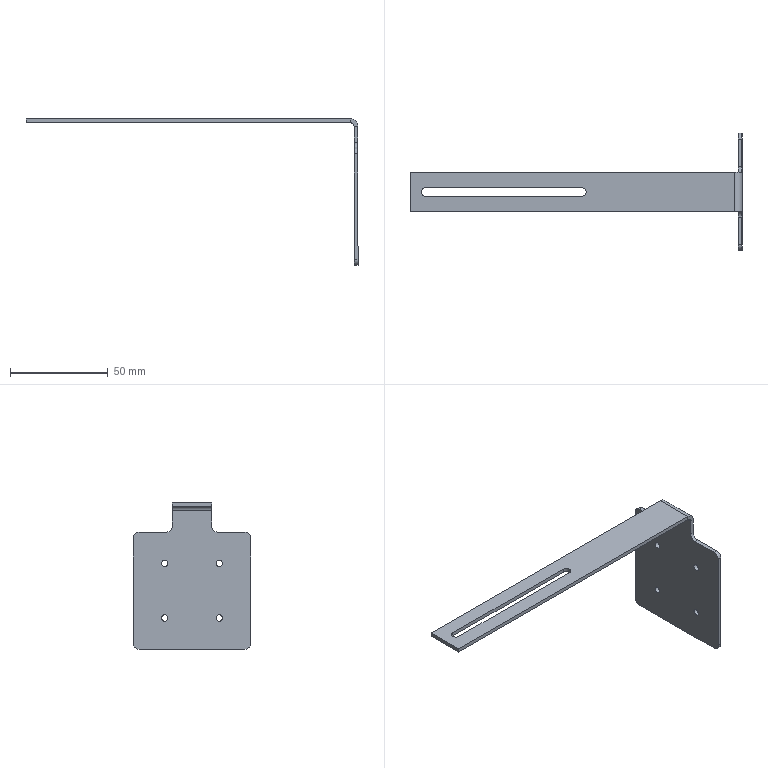Part | STEP file | 1-S938U-100524-012 | 1 solid | 32 faces | box 170 x 60 x 75 mm | volume 13658 mm3 | plane 18 | cylinder 14 | commonest cylinder face diameters 6 x6 3.3 x4 4.4 x2 4 x1 8 x1
STEP:
#1=CARTESIAN_POINT('',(83.,-27.,-13.));
#2=VERTEX_POINT('',#1);
#3=CARTESIAN_POINT('',(83.,-30.,-16.));
#4=VERTEX_POINT('',#3);
#5=CARTESIAN_POINT('',(83.,-27.,-16.));
#6=DIRECTION('',(1.,0.,0.));
#7=DIRECTION('',(0.,-0.7071,0.7071));
#8=AXIS2_PLACEMENT_3D('',#5,#6,#7);
#9=CIRCLE('',#8,3.);
#10=EDGE_CURVE('',#2,#4,#9,.T.);
#11=ORIENTED_EDGE('',*,*,#10,.T.);
#12=CARTESIAN_POINT('',(85.,-30.,-16.));
#13=VERTEX_POINT('',#12);
#14=CARTESIAN_POINT('',(85.,-30.,-16.));
#15=DIRECTION('',(1.,0.,0.));
#16=VECTOR('',#15,10.);
#17=LINE('',#14,#16);
#18=EDGE_CURVE('',#4,#13,#17,.T.);
#19=ORIENTED_EDGE('',*,*,#18,.T.);
#20=CARTESIAN_POINT('',(85.,-27.,-13.));
#21=VERTEX_POINT('',#20);
#22=CARTESIAN_POINT('',(85.,-27.,-16.));
#23=DIRECTION('',(-1.,0.,0.));
#24=DIRECTION('',(0.,-0.7071,0.7071));
#25=AXIS2_PLACEMENT_3D('',#22,#23,#24);
#26=CIRCLE('',#25,3.);
#27=EDGE_CURVE('',#13,#21,#26,.T.);
#28=ORIENTED_EDGE('',*,*,#27,.T.);
#29=CARTESIAN_POINT('',(85.,-27.,-13.));
#30=DIRECTION('',(-1.,0.,0.));
#31=VECTOR('',#30,10.);
#32=LINE('',#29,#31);
#33=EDGE_CURVE('',#21,#2,#32,.T.);
#34=ORIENTED_EDGE('',*,*,#33,.T.);
#35=EDGE_LOOP('',(#11,#19,#28,#34));
#36=FACE_OUTER_BOUND('',#35,.T.);
#37=CARTESIAN_POINT('',(85.,-27.,-16.));
#38=DIRECTION('',(-1.,0.,0.));
#39=DIRECTION('',(0.,-0.7071,0.7071));
#40=AXIS2_PLACEMENT_3D('',#37,#38,#39);
#41=CYLINDRICAL_SURFACE('',#40,3.);
#42=ADVANCED_FACE('',(#36),#41,.T.);
#43=ORIENTED_EDGE('',*,*,#18,.F.);
#44=CARTESIAN_POINT('',(83.,-30.,-70.));
#45=VERTEX_POINT('',#44);
#46=CARTESIAN_POINT('',(83.,-30.,-13.));
#47=DIRECTION('',(0.,0.,-1.));
#48=VECTOR('',#47,10.);
#49=LINE('',#46,#48);
#50=EDGE_CURVE('',#4,#45,#49,.T.);
#51=ORIENTED_EDGE('',*,*,#50,.T.);
#52=CARTESIAN_POINT('',(85.,-30.,-70.));
#53=VERTEX_POINT('',#52);
#54=CARTESIAN_POINT('',(84.,-30.,-70.));
#55=DIRECTION('',(-1.,0.,0.));
#56=VECTOR('',#55,10.);
#57=LINE('',#54,#56);
#58=EDGE_CURVE('',#53,#45,#57,.T.);
#59=ORIENTED_EDGE('',*,*,#58,.F.);
#60=CARTESIAN_POINT('',(85.,-30.,-13.));
#61=DIRECTION('',(0.,0.,-1.));
#62=VECTOR('',#61,10.);
#63=LINE('',#60,#62);
#64=EDGE_CURVE('',#13,#53,#63,.T.);
#65=ORIENTED_EDGE('',*,*,#64,.F.);
#66=EDGE_LOOP('',(#43,#51,#59,#65));
#67=FACE_OUTER_BOUND('',#66,.T.);
#68=CARTESIAN_POINT('',(85.,-30.,-13.));
#69=DIRECTION('',(0.,-1.,0.));
#70=DIRECTION('',(0.,0.,-1.));
#71=AXIS2_PLACEMENT_3D('',#68,#69,#70);
#72=PLANE('',#71);
#73=ADVANCED_FACE('',(#67),#72,.T.);
#74=ORIENTED_EDGE('',*,*,#10,.F.);
#75=CARTESIAN_POINT('',(83.,-13.,-13.));
#76=VERTEX_POINT('',#75);
#77=CARTESIAN_POINT('',(83.,30.,-13.));
#78=DIRECTION('',(0.,-1.,0.));
#79=VECTOR('',#78,10.);
#80=LINE('',#77,#79);
#81=EDGE_CURVE('',#76,#2,#80,.T.);
#82=ORIENTED_EDGE('',*,*,#81,.F.);
#83=CARTESIAN_POINT('',(83.,-10.,-10.));
#84=VERTEX_POINT('',#83);
#85=CARTESIAN_POINT('',(83.,-13.,-10.));
#86=DIRECTION('',(-1.,0.,0.));
#87=DIRECTION('',(0.,0.7071,-0.7071));
#88=AXIS2_PLACEMENT_3D('',#85,#86,#87);
#89=CIRCLE('',#88,3.);
#90=EDGE_CURVE('',#84,#76,#89,.T.);
#91=ORIENTED_EDGE('',*,*,#90,.F.);
#92=CARTESIAN_POINT('',(83.,-10.,-2.));
#93=VERTEX_POINT('',#92);
#94=CARTESIAN_POINT('',(83.,-10.,2.524));
#95=DIRECTION('',(0.,0.,-1.));
#96=VECTOR('',#95,10.);
#97=LINE('',#94,#96);
#98=EDGE_CURVE('',#93,#84,#97,.T.);
#99=ORIENTED_EDGE('',*,*,#98,.F.);
#100=CARTESIAN_POINT('',(83.,10.,-2.));
#101=VERTEX_POINT('',#100);
#102=CARTESIAN_POINT('',(83.,0.,-2.));
#103=DIRECTION('',(0.,1.,0.));
#104=VECTOR('',#103,10.);
#105=LINE('',#102,#104);
#106=EDGE_CURVE('',#93,#101,#105,.T.);
#107=ORIENTED_EDGE('',*,*,#106,.T.);
#108=CARTESIAN_POINT('',(83.,10.,-10.));
#109=VERTEX_POINT('',#108);
#110=CARTESIAN_POINT('',(83.,10.,2.524));
#111=DIRECTION('',(0.,0.,-1.));
#112=VECTOR('',#111,10.);
#113=LINE('',#110,#112);
#114=EDGE_CURVE('',#101,#109,#113,.T.);
#115=ORIENTED_EDGE('',*,*,#114,.T.);
#116=CARTESIAN_POINT('',(83.,13.,-13.));
#117=VERTEX_POINT('',#116);
#118=CARTESIAN_POINT('',(83.,13.,-10.));
#119=DIRECTION('',(-1.,0.,0.));
#120=DIRECTION('',(0.,-0.7071,-0.7071));
#121=AXIS2_PLACEMENT_3D('',#118,#119,#120);
#122=CIRCLE('',#121,3.);
#123=EDGE_CURVE('',#117,#109,#122,.T.);
#124=ORIENTED_EDGE('',*,*,#123,.F.);
#125=CARTESIAN_POINT('',(83.,27.,-13.));
#126=VERTEX_POINT('',#125);
#127=CARTESIAN_POINT('',(83.,30.,-13.));
#128=DIRECTION('',(0.,-1.,0.));
#129=VECTOR('',#128,10.);
#130=LINE('',#127,#129);
#131=EDGE_CURVE('',#126,#117,#130,.T.);
#132=ORIENTED_EDGE('',*,*,#131,.F.);
#133=CARTESIAN_POINT('',(83.,30.,-16.));
#134=VERTEX_POINT('',#133);
#135=CARTESIAN_POINT('',(83.,27.,-16.));
#136=DIRECTION('',(1.,0.,0.));
#137=DIRECTION('',(0.,0.7071,0.7071));
#138=AXIS2_PLACEMENT_3D('',#135,#136,#137);
#139=CIRCLE('',#138,3.);
#140=EDGE_CURVE('',#134,#126,#139,.T.);
#141=ORIENTED_EDGE('',*,*,#140,.F.);
#142=CARTESIAN_POINT('',(83.,30.,-70.));
#143=VERTEX_POINT('',#142);
#144=CARTESIAN_POINT('',(83.,30.,-73.));
#145=DIRECTION('',(0.,0.,1.));
#146=VECTOR('',#145,10.);
#147=LINE('',#144,#146);
#148=EDGE_CURVE('',#143,#134,#147,.T.);
#149=ORIENTED_EDGE('',*,*,#148,.F.);
#150=CARTESIAN_POINT('',(83.,27.,-73.));
#151=VERTEX_POINT('',#150);
#152=CARTESIAN_POINT('',(83.,27.,-70.));
#153=DIRECTION('',(1.,0.,0.));
#154=DIRECTION('',(0.,0.7071,-0.7071));
#155=AXIS2_PLACEMENT_3D('',#152,#153,#154);
#156=CIRCLE('',#155,3.);
#157=EDGE_CURVE('',#151,#143,#156,.T.);
#158=ORIENTED_EDGE('',*,*,#157,.F.);
#159=CARTESIAN_POINT('',(83.,-27.,-73.));
#160=VERTEX_POINT('',#159);
#161=CARTESIAN_POINT('',(83.,-30.,-73.));
#162=DIRECTION('',(0.,1.,0.));
#163=VECTOR('',#162,10.);
#164=LINE('',#161,#163);
#165=EDGE_CURVE('',#160,#151,#164,.T.);
#166=ORIENTED_EDGE('',*,*,#165,.F.);
#167=CARTESIAN_POINT('',(83.,-27.,-70.));
#168=DIRECTION('',(1.,0.,0.));
#169=DIRECTION('',(0.,-0.7071,-0.7071));
#170=AXIS2_PLACEMENT_3D('',#167,#168,#169);
#171=CIRCLE('',#170,3.);
#172=EDGE_CURVE('',#45,#160,#171,.T.);
#173=ORIENTED_EDGE('',*,*,#172,.F.);
#174=ORIENTED_EDGE('',*,*,#50,.F.);
#175=EDGE_LOOP('',(#74,#82,#91,#99,#107,#115,#124,#132,#141,#149,#158,#166,#173,#174));
#176=FACE_OUTER_BOUND('',#175,.T.);
#177=CARTESIAN_POINT('',(83.,14.,-55.35));
#178=VERTEX_POINT('',#177);
#179=CARTESIAN_POINT('',(83.,14.,-57.));
#180=DIRECTION('',(1.,0.,0.));
#181=DIRECTION('',(0.,0.,-1.));
#182=AXIS2_PLACEMENT_3D('',#179,#180,#181);
#183=CIRCLE('',#182,1.65);
#184=EDGE_CURVE('',#178,#178,#183,.T.);
#185=ORIENTED_EDGE('',*,*,#184,.T.);
#186=EDGE_LOOP('',(#185));
#187=FACE_BOUND('',#186,.T.);
#188=CARTESIAN_POINT('',(83.,-14.,-27.35));
#189=VERTEX_POINT('',#188);
#190=CARTESIAN_POINT('',(83.,-14.,-29.));
#191=DIRECTION('',(1.,0.,0.));
#192=DIRECTION('',(0.,0.,-1.));
#193=AXIS2_PLACEMENT_3D('',#190,#191,#192);
#194=CIRCLE('',#193,1.65);
#195=EDGE_CURVE('',#189,#189,#194,.T.);
#196=ORIENTED_EDGE('',*,*,#195,.T.);
#197=EDGE_LOOP('',(#196));
#198=FACE_BOUND('',#197,.T.);
#199=CARTESIAN_POINT('',(83.,14.,-27.35));
#200=VERTEX_POINT('',#199);
#201=CARTESIAN_POINT('',(83.,14.,-29.));
#202=DIRECTION('',(1.,0.,0.));
#203=DIRECTION('',(0.,0.,-1.));
#204=AXIS2_PLACEMENT_3D('',#201,#202,#203);
#205=CIRCLE('',#204,1.65);
#206=EDGE_CURVE('',#200,#200,#205,.T.);
#207=ORIENTED_EDGE('',*,*,#206,.T.);
#208=EDGE_LOOP('',(#207));
#209=FACE_BOUND('',#208,.T.);
#210=CARTESIAN_POINT('',(83.,-14.,-55.35));
#211=VERTEX_POINT('',#210);
#212=CARTESIAN_POINT('',(83.,-14.,-57.));
#213=DIRECTION('',(1.,0.,0.));
#214=DIRECTION('',(0.,0.,-1.));
#215=AXIS2_PLACEMENT_3D('',#212,#213,#214);
#216=CIRCLE('',#215,1.65);
#217=EDGE_CURVE('',#211,#211,#216,.T.);
#218=ORIENTED_EDGE('',*,*,#217,.T.);
#219=EDGE_LOOP('',(#218));
#220=FACE_BOUND('',#219,.T.);
#221=CARTESIAN_POINT('',(83.,0.,-35.238));
#222=DIRECTION('',(1.,0.,0.));
#223=DIRECTION('',(0.,0.,-1.));
#224=AXIS2_PLACEMENT_3D('',#221,#222,#223);
#225=PLANE('',#224);
#226=ADVANCED_FACE('',(#176,#187,#198,#209,#220),#225,.F.);
#227=ORIENTED_EDGE('',*,*,#172,.T.);
#228=CARTESIAN_POINT('',(85.,-27.,-73.));
#229=VERTEX_POINT('',#228);
#230=CARTESIAN_POINT('',(84.,-27.,-73.));
#231=DIRECTION('',(1.,0.,0.));
#232=VECTOR('',#231,10.);
#233=LINE('',#230,#232);
#234=EDGE_CURVE('',#160,#229,#233,.T.);
#235=ORIENTED_EDGE('',*,*,#234,.T.);
#236=CARTESIAN_POINT('',(85.,-27.,-70.));
#237=DIRECTION('',(-1.,0.,0.));
#238=DIRECTION('',(0.,-0.7071,-0.7071));
#239=AXIS2_PLACEMENT_3D('',#236,#237,#238);
#240=CIRCLE('',#239,3.);
#241=EDGE_CURVE('',#229,#53,#240,.T.);
#242=ORIENTED_EDGE('',*,*,#241,.T.);
#243=ORIENTED_EDGE('',*,*,#58,.T.);
#244=EDGE_LOOP('',(#227,#235,#242,#243));
#245=FACE_OUTER_BOUND('',#244,.T.);
#246=CARTESIAN_POINT('',(84.,-27.,-70.));
#247=DIRECTION('',(-1.,0.,0.));
#248=DIRECTION('',(0.,-0.7071,-0.7071));
#249=AXIS2_PLACEMENT_3D('',#246,#247,#248);
#250=CYLINDRICAL_SURFACE('',#249,3.);
#251=ADVANCED_FACE('',(#245),#250,.T.);
#252=ORIENTED_EDGE('',*,*,#234,.F.);
#253=ORIENTED_EDGE('',*,*,#165,.T.);
#254=CARTESIAN_POINT('',(85.,27.,-73.));
#255=VERTEX_POINT('',#254);
#256=CARTESIAN_POINT('',(84.,27.,-73.));
#257=DIRECTION('',(-1.,0.,0.));
#258=VECTOR('',#257,10.);
#259=LINE('',#256,#258);
#260=EDGE_CURVE('',#255,#151,#259,.T.);
#261=ORIENTED_EDGE('',*,*,#260,.F.);
#262=CARTESIAN_POINT('',(85.,-30.,-73.));
#263=DIRECTION('',(0.,1.,0.));
#264=VECTOR('',#263,10.);
#265=LINE('',#262,#264);
#266=EDGE_CURVE('',#229,#255,#265,.T.);
#267=ORIENTED_EDGE('',*,*,#266,.F.);
#268=EDGE_LOOP('',(#252,#253,#261,#267));
#269=FACE_OUTER_BOUND('',#268,.T.);
#270=CARTESIAN_POINT('',(83.,10.,-73.));
#271=DIRECTION('',(0.,0.,-1.));
#272=DIRECTION('',(-1.,0.,0.));
#273=AXIS2_PLACEMENT_3D('',#270,#271,#272);
#274=PLANE('',#273);
#275=ADVANCED_FACE('',(#269),#274,.T.);
#276=ORIENTED_EDGE('',*,*,#157,.T.);
#277=CARTESIAN_POINT('',(85.,30.,-70.));
#278=VERTEX_POINT('',#277);
#279=CARTESIAN_POINT('',(84.,30.,-70.));
#280=DIRECTION('',(1.,0.,0.));
#281=VECTOR('',#280,10.);
#282=LINE('',#279,#281);
#283=EDGE_CURVE('',#143,#278,#282,.T.);
#284=ORIENTED_EDGE('',*,*,#283,.T.);
#285=CARTESIAN_POINT('',(85.,27.,-70.));
#286=DIRECTION('',(-1.,0.,0.));
#287=DIRECTION('',(0.,0.7071,-0.7071));
#288=AXIS2_PLACEMENT_3D('',#285,#286,#287);
#289=CIRCLE('',#288,3.);
#290=EDGE_CURVE('',#278,#255,#289,.T.);
#291=ORIENTED_EDGE('',*,*,#290,.T.);
#292=ORIENTED_EDGE('',*,*,#260,.T.);
#293=EDGE_LOOP('',(#276,#284,#291,#292));
#294=FACE_OUTER_BOUND('',#293,.T.);
#295=CARTESIAN_POINT('',(84.,27.,-70.));
#296=DIRECTION('',(-1.,0.,0.));
#297=DIRECTION('',(0.,0.7071,-0.7071));
#298=AXIS2_PLACEMENT_3D('',#295,#296,#297);
#299=CYLINDRICAL_SURFACE('',#298,3.);
#300=ADVANCED_FACE('',(#294),#299,.T.);
#301=ORIENTED_EDGE('',*,*,#283,.F.);
#302=ORIENTED_EDGE('',*,*,#148,.T.);
#303=CARTESIAN_POINT('',(85.,30.,-16.));
#304=VERTEX_POINT('',#303);
#305=CARTESIAN_POINT('',(85.,30.,-16.));
#306=DIRECTION('',(-1.,0.,0.));
#307=VECTOR('',#306,10.);
#308=LINE('',#305,#307);
#309=EDGE_CURVE('',#304,#134,#308,.T.);
#310=ORIENTED_EDGE('',*,*,#309,.F.);
#311=CARTESIAN_POINT('',(85.,30.,-73.));
#312=DIRECTION('',(0.,0.,1.));
#313=VECTOR('',#312,10.);
#314=LINE('',#311,#313);
#315=EDGE_CURVE('',#278,#304,#314,.T.);
#316=ORIENTED_EDGE('',*,*,#315,.F.);
#317=EDGE_LOOP('',(#301,#302,#310,#316));
#318=FACE_OUTER_BOUND('',#317,.T.);
#319=CARTESIAN_POINT('',(85.,30.,-73.));
#320=DIRECTION('',(0.,1.,0.));
#321=DIRECTION('',(0.,0.,1.));
#322=AXIS2_PLACEMENT_3D('',#319,#320,#321);
#323=PLANE('',#322);
#324=ADVANCED_FACE('',(#318),#323,.T.);
#325=ORIENTED_EDGE('',*,*,#140,.T.);
#326=CARTESIAN_POINT('',(85.,27.,-13.));
#327=VERTEX_POINT('',#326);
#328=CARTESIAN_POINT('',(85.,27.,-13.));
#329=DIRECTION('',(1.,0.,0.));
#330=VECTOR('',#329,10.);
#331=LINE('',#328,#330);
#332=EDGE_CURVE('',#126,#327,#331,.T.);
#333=ORIENTED_EDGE('',*,*,#332,.T.);
#334=CARTESIAN_POINT('',(85.,27.,-16.));
#335=DIRECTION('',(-1.,0.,0.));
#336=DIRECTION('',(0.,0.7071,0.7071));
#337=AXIS2_PLACEMENT_3D('',#334,#335,#336);
#338=CIRCLE('',#337,3.);
#339=EDGE_CURVE('',#327,#304,#338,.T.);
#340=ORIENTED_EDGE('',*,*,#339,.T.);
#341=ORIENTED_EDGE('',*,*,#309,.T.);
#342=EDGE_LOOP('',(#325,#333,#340,#341));
#343=FACE_OUTER_BOUND('',#342,.T.);
#344=CARTESIAN_POINT('',(85.,27.,-16.));
#345=DIRECTION('',(-1.,0.,0.));
#346=DIRECTION('',(0.,0.7071,0.7071));
#347=AXIS2_PLACEMENT_3D('',#344,#345,#346);
#348=CYLINDRICAL_SURFACE('',#347,3.);
#349=ADVANCED_FACE('',(#343),#348,.T.);
#350=ORIENTED_EDGE('',*,*,#90,.T.);
#351=CARTESIAN_POINT('',(85.,-13.,-13.));
#352=VERTEX_POINT('',#351);
#353=CARTESIAN_POINT('',(84.,-13.,-13.));
#354=DIRECTION('',(1.,0.,0.));
#355=VECTOR('',#354,10.);
#356=LINE('',#353,#355);
#357=EDGE_CURVE('',#76,#352,#356,.T.);
#358=ORIENTED_EDGE('',*,*,#357,.T.);
#359=CARTESIAN_POINT('',(85.,-10.,-10.));
#360=VERTEX_POINT('',#359);
#361=CARTESIAN_POINT('',(85.,-13.,-10.));
#362=DIRECTION('',(1.,0.,0.));
#363=DIRECTION('',(0.,0.7071,-0.7071));
#364=AXIS2_PLACEMENT_3D('',#361,#362,#363);
#365=CIRCLE('',#364,3.);
#366=EDGE_CURVE('',#352,#360,#365,.T.);
#367=ORIENTED_EDGE('',*,*,#366,.T.);
#368=CARTESIAN_POINT('',(84.,-10.,-10.));
#369=DIRECTION('',(-1.,0.,0.));
#370=VECTOR('',#369,10.);
#371=LINE('',#368,#370);
#372=EDGE_CURVE('',#360,#84,#371,.T.);
#373=ORIENTED_EDGE('',*,*,#372,.T.);
#374=EDGE_LOOP('',(#350,#358,#367,#373));
#375=FACE_OUTER_BOUND('',#374,.T.);
#376=CARTESIAN_POINT('',(84.,-13.,-10.));
#377=DIRECTION('',(1.,0.,0.));
#378=DIRECTION('',(0.,0.7071,-0.7071));
#379=AXIS2_PLACEMENT_3D('',#376,#377,#378);
#380=CYLINDRICAL_SURFACE('',#379,3.);
#381=ADVANCED_FACE('',(#375),#380,.F.);
#382=ORIENTED_EDGE('',*,*,#33,.F.);
#383=CARTESIAN_POINT('',(85.,30.,-13.));
#384=DIRECTION('',(0.,-1.,0.));
#385=VECTOR('',#384,10.);
#386=LINE('',#383,#385);
#387=EDGE_CURVE('',#352,#21,#386,.T.);
#388=ORIENTED_EDGE('',*,*,#387,.F.);
#389=ORIENTED_EDGE('',*,*,#357,.F.);
#390=ORIENTED_EDGE('',*,*,#81,.T.);
#391=EDGE_LOOP('',(#382,#388,#389,#390));
#392=FACE_OUTER_BOUND('',#391,.T.);
#393=CARTESIAN_POINT('',(85.,30.,-13.));
#394=DIRECTION('',(0.,0.,1.));
#395=DIRECTION('',(1.,0.,0.));
#396=AXIS2_PLACEMENT_3D('',#393,#394,#395);
#397=PLANE('',#396);
#398=ADVANCED_FACE('',(#392),#397,.T.);
#399=CARTESIAN_POINT('',(85.,10.,-10.));
#400=VERTEX_POINT('',#399);
#401=CARTESIAN_POINT('',(85.,13.,-13.));
#402=VERTEX_POINT('',#401);
#403=CARTESIAN_POINT('',(85.,13.,-10.));
#404=DIRECTION('',(1.,0.,0.));
#405=DIRECTION('',(0.,-0.7071,-0.7071));
#406=AXIS2_PLACEMENT_3D('',#403,#404,#405);
#407=CIRCLE('',#406,3.);
#408=EDGE_CURVE('',#400,#402,#407,.T.);
#409=ORIENTED_EDGE('',*,*,#408,.T.);
#410=CARTESIAN_POINT('',(84.,13.,-13.));
#411=DIRECTION('',(-1.,0.,0.));
#412=VECTOR('',#411,10.);
#413=LINE('',#410,#412);
#414=EDGE_CURVE('',#402,#117,#413,.T.);
#415=ORIENTED_EDGE('',*,*,#414,.T.);
#416=ORIENTED_EDGE('',*,*,#123,.T.);
#417=CARTESIAN_POINT('',(84.,10.,-10.));
#418=DIRECTION('',(1.,0.,0.));
#419=VECTOR('',#418,10.);
#420=LINE('',#417,#419);
#421=EDGE_CURVE('',#109,#400,#420,.T.);
#422=ORIENTED_EDGE('',*,*,#421,.T.);
#423=EDGE_LOOP('',(#409,#415,#416,#422));
#424=FACE_OUTER_BOUND('',#423,.T.);
#425=CARTESIAN_POINT('',(84.,13.,-10.));
#426=DIRECTION('',(-1.,0.,0.));
#427=DIRECTION('',(0.,-0.7071,-0.7071));
#428=AXIS2_PLACEMENT_3D('',#425,#426,#427);
#429=CYLINDRICAL_SURFACE('',#428,3.);
#430=ADVANCED_FACE('',(#424),#429,.F.);
#431=ORIENTED_EDGE('',*,*,#332,.F.);
#432=ORIENTED_EDGE('',*,*,#131,.T.);
#433=ORIENTED_EDGE('',*,*,#414,.F.);
#434=CARTESIAN_POINT('',(85.,30.,-13.));
#435=DIRECTION('',(0.,-1.,0.));
#436=VECTOR('',#435,10.);
#437=LINE('',#434,#436);
#438=EDGE_CURVE('',#327,#402,#437,.T.);
#439=ORIENTED_EDGE('',*,*,#438,.F.);
#440=EDGE_LOOP('',(#431,#432,#433,#439));
#441=FACE_OUTER_BOUND('',#440,.T.);
#442=CARTESIAN_POINT('',(85.,30.,-13.));
#443=DIRECTION('',(0.,0.,1.));
#444=DIRECTION('',(1.,0.,0.));
#445=AXIS2_PLACEMENT_3D('',#442,#443,#444);
#446=PLANE('',#445);
#447=ADVANCED_FACE('',(#441),#446,.T.);
#448=ORIENTED_EDGE('',*,*,#184,.F.);
#449=CARTESIAN_POINT('',(85.,14.,-55.35));
#450=VERTEX_POINT('',#449);
#451=CARTESIAN_POINT('',(79.1,14.,-55.35));
#452=DIRECTION('',(1.,0.,0.));
#453=VECTOR('',#452,1.65);
#454=LINE('',#451,#453);
#455=EDGE_CURVE('',#178,#450,#454,.T.);
#456=ORIENTED_EDGE('',*,*,#455,.T.);
#457=CARTESIAN_POINT('',(85.,14.,-58.65));
#458=VERTEX_POINT('',#457);
#459=CARTESIAN_POINT('',(85.,14.,-57.));
#460=DIRECTION('',(-1.,0.,0.));
#461=DIRECTION('',(0.,0.,-1.));
#462=AXIS2_PLACEMENT_3D('',#459,#460,#461);
#463=CIRCLE('',#462,1.65);
#464=EDGE_CURVE('',#458,#450,#463,.T.);
#465=ORIENTED_EDGE('',*,*,#464,.F.);
#466=CARTESIAN_POINT('',(85.,14.,-57.));
#467=DIRECTION('',(-1.,0.,0.));
#468=DIRECTION('',(0.,0.,-1.));
#469=AXIS2_PLACEMENT_3D('',#466,#467,#468);
#470=CIRCLE('',#469,1.65);
#471=EDGE_CURVE('',#450,#458,#470,.T.);
#472=ORIENTED_EDGE('',*,*,#471,.F.);
#473=ORIENTED_EDGE('',*,*,#455,.F.);
#474=EDGE_LOOP('',(#448,#456,#465,#472,#473));
#475=FACE_OUTER_BOUND('',#474,.T.);
#476=CARTESIAN_POINT('',(79.1,14.,-57.));
#477=DIRECTION('',(1.,0.,0.));
#478=DIRECTION('',(0.,0.,-1.));
#479=AXIS2_PLACEMENT_3D('',#476,#477,#478);
#480=CYLINDRICAL_SURFACE('',#479,1.65);
#481=ADVANCED_FACE('',(#475),#480,.F.);
#482=ORIENTED_EDGE('',*,*,#195,.F.);
#483=CARTESIAN_POINT('',(85.,-14.,-27.35));
#484=VERTEX_POINT('',#483);
#485=CARTESIAN_POINT('',(79.1,-14.,-27.35));
#486=DIRECTION('',(1.,0.,0.));
#487=VECTOR('',#486,1.65);
#488=LINE('',#485,#487);
#489=EDGE_CURVE('',#189,#484,#488,.T.);
#490=ORIENTED_EDGE('',*,*,#489,.T.);
#491=CARTESIAN_POINT('',(85.,-14.,-30.65));
#492=VERTEX_POINT('',#491);
#493=CARTESIAN_POINT('',(85.,-14.,-29.));
#494=DIRECTION('',(-1.,0.,0.));
#495=DIRECTION('',(0.,0.,-1.));
#496=AXIS2_PLACEMENT_3D('',#493,#494,#495);
#497=CIRCLE('',#496,1.65);
#498=EDGE_CURVE('',#492,#484,#497,.T.);
#499=ORIENTED_EDGE('',*,*,#498,.F.);
#500=CARTESIAN_POINT('',(85.,-14.,-29.));
#501=DIRECTION('',(-1.,0.,0.));
#502=DIRECTION('',(0.,0.,-1.));
#503=AXIS2_PLACEMENT_3D('',#500,#501,#502);
#504=CIRCLE('',#503,1.65);
#505=EDGE_CURVE('',#484,#492,#504,.T.);
#506=ORIENTED_EDGE('',*,*,#505,.F.);
#507=ORIENTED_EDGE('',*,*,#489,.F.);
#508=EDGE_LOOP('',(#482,#490,#499,#506,#507));
#509=FACE_OUTER_BOUND('',#508,.T.);
#510=CARTESIAN_POINT('',(79.1,-14.,-29.));
#511=DIRECTION('',(1.,0.,0.));
#512=DIRECTION('',(0.,0.,-1.));
#513=AXIS2_PLACEMENT_3D('',#510,#511,#512);
#514=CYLINDRICAL_SURFACE('',#513,1.65);
#515=ADVANCED_FACE('',(#509),#514,.F.);
#516=ORIENTED_EDGE('',*,*,#206,.F.);
#517=CARTESIAN_POINT('',(85.,14.,-27.35));
#518=VERTEX_POINT('',#517);
#519=CARTESIAN_POINT('',(79.1,14.,-27.35));
#520=DIRECTION('',(1.,0.,0.));
#521=VECTOR('',#520,1.65);
#522=LINE('',#519,#521);
#523=EDGE_CURVE('',#200,#518,#522,.T.);
#524=ORIENTED_EDGE('',*,*,#523,.T.);
#525=CARTESIAN_POINT('',(85.,14.,-30.65));
#526=VERTEX_POINT('',#525);
#527=CARTESIAN_POINT('',(85.,14.,-29.));
#528=DIRECTION('',(-1.,0.,0.));
#529=DIRECTION('',(0.,0.,-1.));
#530=AXIS2_PLACEMENT_3D('',#527,#528,#529);
#531=CIRCLE('',#530,1.65);
#532=EDGE_CURVE('',#526,#518,#531,.T.);
#533=ORIENTED_EDGE('',*,*,#532,.F.);
#534=CARTESIAN_POINT('',(85.,14.,-29.));
#535=DIRECTION('',(-1.,0.,0.));
#536=DIRECTION('',(0.,0.,-1.));
#537=AXIS2_PLACEMENT_3D('',#534,#535,#536);
#538=CIRCLE('',#537,1.65);
#539=EDGE_CURVE('',#518,#526,#538,.T.);
#540=ORIENTED_EDGE('',*,*,#539,.F.);
#541=ORIENTED_EDGE('',*,*,#523,.F.);
#542=EDGE_LOOP('',(#516,#524,#533,#540,#541));
#543=FACE_OUTER_BOUND('',#542,.T.);
#544=CARTESIAN_POINT('',(79.1,14.,-29.));
#545=DIRECTION('',(1.,0.,0.));
#546=DIRECTION('',(0.,0.,-1.));
#547=AXIS2_PLACEMENT_3D('',#544,#545,#546);
#548=CYLINDRICAL_SURFACE('',#547,1.65);
#549=ADVANCED_FACE('',(#543),#548,.F.);
#550=ORIENTED_EDGE('',*,*,#217,.F.);
#551=CARTESIAN_POINT('',(85.,-14.,-55.35));
#552=VERTEX_POINT('',#551);
#553=CARTESIAN_POINT('',(79.1,-14.,-55.35));
#554=DIRECTION('',(1.,0.,0.));
#555=VECTOR('',#554,1.65);
#556=LINE('',#553,#555);
#557=EDGE_CURVE('',#211,#552,#556,.T.);
#558=ORIENTED_EDGE('',*,*,#557,.T.);
#559=CARTESIAN_POINT('',(85.,-14.,-58.65));
#560=VERTEX_POINT('',#559);
#561=CARTESIAN_POINT('',(85.,-14.,-57.));
#562=DIRECTION('',(-1.,0.,0.));
#563=DIRECTION('',(0.,0.,-1.));
#564=AXIS2_PLACEMENT_3D('',#561,#562,#563);
#565=CIRCLE('',#564,1.65);
#566=EDGE_CURVE('',#560,#552,#565,.T.);
#567=ORIENTED_EDGE('',*,*,#566,.F.);
#568=CARTESIAN_POINT('',(85.,-14.,-57.));
#569=DIRECTION('',(-1.,0.,0.));
#570=DIRECTION('',(0.,0.,-1.));
#571=AXIS2_PLACEMENT_3D('',#568,#569,#570);
#572=CIRCLE('',#571,1.65);
#573=EDGE_CURVE('',#552,#560,#572,.T.);
#574=ORIENTED_EDGE('',*,*,#573,.F.);
#575=ORIENTED_EDGE('',*,*,#557,.F.);
#576=EDGE_LOOP('',(#550,#558,#567,#574,#575));
#577=FACE_OUTER_BOUND('',#576,.T.);
#578=CARTESIAN_POINT('',(79.1,-14.,-57.));
#579=DIRECTION('',(1.,0.,0.));
#580=DIRECTION('',(0.,0.,-1.));
#581=AXIS2_PLACEMENT_3D('',#578,#579,#580);
#582=CYLINDRICAL_SURFACE('',#581,1.65);
#583=ADVANCED_FACE('',(#577),#582,.F.);
#584=ORIENTED_EDGE('',*,*,#421,.F.);
#585=ORIENTED_EDGE('',*,*,#114,.F.);
#586=CARTESIAN_POINT('',(85.,10.,-2.));
#587=VERTEX_POINT('',#586);
#588=CARTESIAN_POINT('',(83.44,10.,-2.));
#589=DIRECTION('',(1.,0.,0.));
#590=VECTOR('',#589,10.);
#591=LINE('',#588,#590);
#592=EDGE_CURVE('',#101,#587,#591,.T.);
#593=ORIENTED_EDGE('',*,*,#592,.T.);
#594=CARTESIAN_POINT('',(85.,10.,-2.));
#595=DIRECTION('',(0.,0.,-1.));
#596=VECTOR('',#595,10.);
#597=LINE('',#594,#596);
#598=EDGE_CURVE('',#587,#400,#597,.T.);
#599=ORIENTED_EDGE('',*,*,#598,.T.);
#600=EDGE_LOOP('',(#584,#585,#593,#599));
#601=FACE_OUTER_BOUND('',#600,.T.);
#602=CARTESIAN_POINT('',(83.,10.,-2.));
#603=DIRECTION('',(0.,1.,0.));
#604=DIRECTION('',(1.,0.,0.));
#605=AXIS2_PLACEMENT_3D('',#602,#603,#604);
#606=PLANE('',#605);
#607=ADVANCED_FACE('',(#601),#606,.T.);
#608=CARTESIAN_POINT('',(3.,2.2,0.));
#609=VERTEX_POINT('',#608);
#610=CARTESIAN_POINT('',(-77.,2.2,0.));
#611=VERTEX_POINT('',#610);
#612=CARTESIAN_POINT('',(-38.5,2.2,0.));
#613=DIRECTION('',(-1.,0.,0.));
#614=VECTOR('',#613,10.);
#615=LINE('',#612,#614);
#616=EDGE_CURVE('',#609,#611,#615,.T.);
#617=ORIENTED_EDGE('',*,*,#616,.F.);
#618=CARTESIAN_POINT('',(3.,2.2,2.));
#619=VERTEX_POINT('',#618);
#620=CARTESIAN_POINT('',(3.,2.2,2.));
#621=DIRECTION('',(0.,0.,-1.));
#622=VECTOR('',#621,10.);
#623=LINE('',#620,#622);
#624=EDGE_CURVE('',#619,#609,#623,.T.);
#625=ORIENTED_EDGE('',*,*,#624,.F.);
#626=CARTESIAN_POINT('',(-77.,2.2,2.));
#627=VERTEX_POINT('',#626);
#628=CARTESIAN_POINT('',(-38.5,2.2,2.));
#629=DIRECTION('',(1.,0.,0.));
#630=VECTOR('',#629,10.);
#631=LINE('',#628,#630);
#632=EDGE_CURVE('',#627,#619,#631,.T.);
#633=ORIENTED_EDGE('',*,*,#632,.F.);
#634=CARTESIAN_POINT('',(-77.,2.2,2.));
#635=DIRECTION('',(0.,0.,-1.));
#636=VECTOR('',#635,10.);
#637=LINE('',#634,#636);
#638=EDGE_CURVE('',#627,#611,#637,.T.);
#639=ORIENTED_EDGE('',*,*,#638,.T.);
#640=EDGE_LOOP('',(#617,#625,#633,#639));
#641=FACE_OUTER_BOUND('',#640,.T.);
#642=CARTESIAN_POINT('',(-77.,2.2,2.));
#643=DIRECTION('',(0.,1.,0.));
#644=DIRECTION('',(1.,0.,0.));
#645=AXIS2_PLACEMENT_3D('',#642,#643,#644);
#646=PLANE('',#645);
#647=ADVANCED_FACE('',(#641),#646,.F.);
#648=CARTESIAN_POINT('',(-77.,-2.2,0.));
#649=VERTEX_POINT('',#648);
#650=CARTESIAN_POINT('',(-77.,0.,0.));
#651=DIRECTION('',(0.,0.,1.));
#652=DIRECTION('',(0.,1.,0.));
#653=AXIS2_PLACEMENT_3D('',#650,#651,#652);
#654=CIRCLE('',#653,2.2);
#655=EDGE_CURVE('',#611,#649,#654,.T.);
#656=ORIENTED_EDGE('',*,*,#655,.F.);
#657=ORIENTED_EDGE('',*,*,#638,.F.);
#658=CARTESIAN_POINT('',(-77.,-2.2,2.));
#659=VERTEX_POINT('',#658);
#660=CARTESIAN_POINT('',(-77.,0.,2.));
#661=DIRECTION('',(0.,0.,-1.));
#662=DIRECTION('',(0.,1.,0.));
#663=AXIS2_PLACEMENT_3D('',#660,#661,#662);
#664=CIRCLE('',#663,2.2);
#665=EDGE_CURVE('',#659,#627,#664,.T.);
#666=ORIENTED_EDGE('',*,*,#665,.F.);
#667=CARTESIAN_POINT('',(-77.,-2.2,2.));
#668=DIRECTION('',(0.,0.,-1.));
#669=VECTOR('',#668,10.);
#670=LINE('',#667,#669);
#671=EDGE_CURVE('',#659,#649,#670,.T.);
#672=ORIENTED_EDGE('',*,*,#671,.T.);
#673=EDGE_LOOP('',(#656,#657,#666,#672));
#674=FACE_OUTER_BOUND('',#673,.T.);
#675=CARTESIAN_POINT('',(-77.,0.,2.));
#676=DIRECTION('',(0.,0.,-1.));
#677=DIRECTION('',(0.,1.,0.));
#678=AXIS2_PLACEMENT_3D('',#675,#676,#677);
#679=CYLINDRICAL_SURFACE('',#678,2.2);
#680=ADVANCED_FACE('',(#674),#679,.F.);
#681=CARTESIAN_POINT('',(3.,-2.2,0.));
#682=VERTEX_POINT('',#681);
#683=CARTESIAN_POINT('',(1.5,-2.2,0.));
#684=DIRECTION('',(1.,0.,0.));
#685=VECTOR('',#684,10.);
#686=LINE('',#683,#685);
#687=EDGE_CURVE('',#649,#682,#686,.T.);
#688=ORIENTED_EDGE('',*,*,#687,.F.);
#689=ORIENTED_EDGE('',*,*,#671,.F.);
#690=CARTESIAN_POINT('',(3.,-2.2,2.));
#691=VERTEX_POINT('',#690);
#692=CARTESIAN_POINT('',(1.5,-2.2,2.));
#693=DIRECTION('',(-1.,0.,0.));
#694=VECTOR('',#693,10.);
#695=LINE('',#692,#694);
#696=EDGE_CURVE('',#691,#659,#695,.T.);
#697=ORIENTED_EDGE('',*,*,#696,.F.);
#698=CARTESIAN_POINT('',(3.,-2.2,2.));
#699=DIRECTION('',(0.,0.,-1.));
#700=VECTOR('',#699,10.);
#701=LINE('',#698,#700);
#702=EDGE_CURVE('',#691,#682,#701,.T.);
#703=ORIENTED_EDGE('',*,*,#702,.T.);
#704=EDGE_LOOP('',(#688,#689,#697,#703));
#705=FACE_OUTER_BOUND('',#704,.T.);
#706=CARTESIAN_POINT('',(3.,-2.2,2.));
#707=DIRECTION('',(0.,-1.,0.));
#708=DIRECTION('',(-1.,0.,0.));
#709=AXIS2_PLACEMENT_3D('',#706,#707,#708);
#710=PLANE('',#709);
#711=ADVANCED_FACE('',(#705),#710,.F.);
#712=CARTESIAN_POINT('',(3.,0.,0.));
#713=DIRECTION('',(0.,0.,1.));
#714=DIRECTION('',(0.,-1.,0.));
#715=AXIS2_PLACEMENT_3D('',#712,#713,#714);
#716=CIRCLE('',#715,2.2);
#717=EDGE_CURVE('',#682,#609,#716,.T.);
#718=ORIENTED_EDGE('',*,*,#717,.F.);
#719=ORIENTED_EDGE('',*,*,#702,.F.);
#720=CARTESIAN_POINT('',(3.,0.,2.));
#721=DIRECTION('',(0.,0.,-1.));
#722=DIRECTION('',(0.,-1.,0.));
#723=AXIS2_PLACEMENT_3D('',#720,#721,#722);
#724=CIRCLE('',#723,2.2);
#725=EDGE_CURVE('',#619,#691,#724,.T.);
#726=ORIENTED_EDGE('',*,*,#725,.F.);
#727=ORIENTED_EDGE('',*,*,#624,.T.);
#728=EDGE_LOOP('',(#718,#719,#726,#727));
#729=FACE_OUTER_BOUND('',#728,.T.);
#730=CARTESIAN_POINT('',(3.,0.,2.));
#731=DIRECTION('',(0.,0.,-1.));
#732=DIRECTION('',(0.,-1.,0.));
#733=AXIS2_PLACEMENT_3D('',#730,#731,#732);
#734=CYLINDRICAL_SURFACE('',#733,2.2);
#735=ADVANCED_FACE('',(#729),#734,.F.);
#736=CARTESIAN_POINT('',(85.,-10.,-2.));
#737=VERTEX_POINT('',#736);
#738=CARTESIAN_POINT('',(85.,0.,-2.));
#739=DIRECTION('',(0.,-1.,0.));
#740=VECTOR('',#739,10.);
#741=LINE('',#738,#740);
#742=EDGE_CURVE('',#587,#737,#741,.T.);
#743=ORIENTED_EDGE('',*,*,#742,.F.);
#744=CARTESIAN_POINT('',(81.,10.,2.));
#745=VERTEX_POINT('',#744);
#746=CARTESIAN_POINT('',(81.,10.,-2.));
#747=DIRECTION('',(0.,1.,0.));
#748=DIRECTION('',(0.,0.,1.));
#749=AXIS2_PLACEMENT_3D('',#746,#747,#748);
#750=CIRCLE('',#749,4.);
#751=EDGE_CURVE('',#745,#587,#750,.T.);
#752=ORIENTED_EDGE('',*,*,#751,.F.);
#753=CARTESIAN_POINT('',(81.,-10.,2.));
#754=VERTEX_POINT('',#753);
#755=CARTESIAN_POINT('',(81.,-5.,2.));
#756=DIRECTION('',(0.,1.,0.));
#757=VECTOR('',#756,10.);
#758=LINE('',#755,#757);
#759=EDGE_CURVE('',#754,#745,#758,.T.);
#760=ORIENTED_EDGE('',*,*,#759,.F.);
#761=CARTESIAN_POINT('',(81.,-10.,-2.));
#762=DIRECTION('',(0.,-1.,0.));
#763=DIRECTION('',(1.,0.,0.));
#764=AXIS2_PLACEMENT_3D('',#761,#762,#763);
#765=CIRCLE('',#764,4.);
#766=EDGE_CURVE('',#737,#754,#765,.T.);
#767=ORIENTED_EDGE('',*,*,#766,.F.);
#768=EDGE_LOOP('',(#743,#752,#760,#767));
#769=FACE_OUTER_BOUND('',#768,.T.);
#770=CARTESIAN_POINT('',(81.,0.,-2.));
#771=DIRECTION('',(0.,1.,0.));
#772=DIRECTION('',(0.,0.,1.));
#773=AXIS2_PLACEMENT_3D('',#770,#771,#772);
#774=CYLINDRICAL_SURFACE('',#773,4.);
#775=ADVANCED_FACE('',(#769),#774,.T.);
#776=ORIENTED_EDGE('',*,*,#372,.F.);
#777=CARTESIAN_POINT('',(85.,-10.,2.524));
#778=DIRECTION('',(0.,0.,1.));
#779=VECTOR('',#778,10.);
#780=LINE('',#777,#779);
#781=EDGE_CURVE('',#360,#737,#780,.T.);
#782=ORIENTED_EDGE('',*,*,#781,.T.);
#783=CARTESIAN_POINT('',(83.44,-10.,-2.));
#784=DIRECTION('',(-1.,0.,0.));
#785=VECTOR('',#784,10.);
#786=LINE('',#783,#785);
#787=EDGE_CURVE('',#737,#93,#786,.T.);
#788=ORIENTED_EDGE('',*,*,#787,.T.);
#789=ORIENTED_EDGE('',*,*,#98,.T.);
#790=EDGE_LOOP('',(#776,#782,#788,#789));
#791=FACE_OUTER_BOUND('',#790,.T.);
#792=CARTESIAN_POINT('',(83.,-10.,-2.));
#793=DIRECTION('',(0.,-1.,0.));
#794=DIRECTION('',(-1.,0.,0.));
#795=AXIS2_PLACEMENT_3D('',#792,#793,#794);
#796=PLANE('',#795);
#797=ADVANCED_FACE('',(#791),#796,.T.);
#798=ORIENTED_EDGE('',*,*,#592,.F.);
#799=CARTESIAN_POINT('',(81.,10.,0.));
#800=VERTEX_POINT('',#799);
#801=CARTESIAN_POINT('',(81.,10.,-2.));
#802=DIRECTION('',(0.,1.,0.));
#803=DIRECTION('',(0.,0.,1.));
#804=AXIS2_PLACEMENT_3D('',#801,#802,#803);
#805=CIRCLE('',#804,2.);
#806=EDGE_CURVE('',#800,#101,#805,.T.);
#807=ORIENTED_EDGE('',*,*,#806,.F.);
#808=CARTESIAN_POINT('',(81.,10.,0.));
#809=DIRECTION('',(0.,0.,-1.));
#810=VECTOR('',#809,10.);
#811=LINE('',#808,#810);
#812=EDGE_CURVE('',#745,#800,#811,.T.);
#813=ORIENTED_EDGE('',*,*,#812,.F.);
#814=ORIENTED_EDGE('',*,*,#751,.T.);
#815=EDGE_LOOP('',(#798,#807,#813,#814));
#816=FACE_OUTER_BOUND('',#815,.T.);
#817=CARTESIAN_POINT('',(83.,10.,-2.));
#818=DIRECTION('',(0.,1.,0.));
#819=DIRECTION('',(0.,0.,1.));
#820=AXIS2_PLACEMENT_3D('',#817,#818,#819);
#821=PLANE('',#820);
#822=ADVANCED_FACE('',(#816),#821,.T.);
#823=ORIENTED_EDGE('',*,*,#787,.F.);
#824=ORIENTED_EDGE('',*,*,#766,.T.);
#825=CARTESIAN_POINT('',(81.,-10.,0.));
#826=VERTEX_POINT('',#825);
#827=CARTESIAN_POINT('',(81.,-10.,0.));
#828=DIRECTION('',(0.,0.,1.));
#829=VECTOR('',#828,10.);
#830=LINE('',#827,#829);
#831=EDGE_CURVE('',#826,#754,#830,.T.);
#832=ORIENTED_EDGE('',*,*,#831,.F.);
#833=CARTESIAN_POINT('',(81.,-10.,-2.));
#834=DIRECTION('',(0.,1.,0.));
#835=DIRECTION('',(0.,0.,1.));
#836=AXIS2_PLACEMENT_3D('',#833,#834,#835);
#837=CIRCLE('',#836,2.);
#838=EDGE_CURVE('',#826,#93,#837,.T.);
#839=ORIENTED_EDGE('',*,*,#838,.T.);
#840=EDGE_LOOP('',(#823,#824,#832,#839));
#841=FACE_OUTER_BOUND('',#840,.T.);
#842=CARTESIAN_POINT('',(85.,-10.,-2.));
#843=DIRECTION('',(0.,-1.,0.));
#844=DIRECTION('',(0.,0.,-1.));
#845=AXIS2_PLACEMENT_3D('',#842,#843,#844);
#846=PLANE('',#845);
#847=ADVANCED_FACE('',(#841),#846,.T.);
#848=ORIENTED_EDGE('',*,*,#27,.F.);
#849=ORIENTED_EDGE('',*,*,#64,.T.);
#850=ORIENTED_EDGE('',*,*,#241,.F.);
#851=ORIENTED_EDGE('',*,*,#266,.T.);
#852=ORIENTED_EDGE('',*,*,#290,.F.);
#853=ORIENTED_EDGE('',*,*,#315,.T.);
#854=ORIENTED_EDGE('',*,*,#339,.F.);
#855=ORIENTED_EDGE('',*,*,#438,.T.);
#856=ORIENTED_EDGE('',*,*,#408,.F.);
#857=ORIENTED_EDGE('',*,*,#598,.F.);
#858=ORIENTED_EDGE('',*,*,#742,.T.);
#859=ORIENTED_EDGE('',*,*,#781,.F.);
#860=ORIENTED_EDGE('',*,*,#366,.F.);
#861=ORIENTED_EDGE('',*,*,#387,.T.);
#862=EDGE_LOOP('',(#848,#849,#850,#851,#852,#853,#854,#855,#856,#857,#858,#859,#860,#861));
#863=FACE_OUTER_BOUND('',#862,.T.);
#864=ORIENTED_EDGE('',*,*,#464,.T.);
#865=ORIENTED_EDGE('',*,*,#471,.T.);
#866=EDGE_LOOP('',(#864,#865));
#867=FACE_BOUND('',#866,.T.);
#868=ORIENTED_EDGE('',*,*,#498,.T.);
#869=ORIENTED_EDGE('',*,*,#505,.T.);
#870=EDGE_LOOP('',(#868,#869));
#871=FACE_BOUND('',#870,.T.);
#872=ORIENTED_EDGE('',*,*,#532,.T.);
#873=ORIENTED_EDGE('',*,*,#539,.T.);
#874=EDGE_LOOP('',(#872,#873));
#875=FACE_BOUND('',#874,.T.);
#876=ORIENTED_EDGE('',*,*,#566,.T.);
#877=ORIENTED_EDGE('',*,*,#573,.T.);
#878=EDGE_LOOP('',(#876,#877));
#879=FACE_BOUND('',#878,.T.);
#880=CARTESIAN_POINT('',(85.,0.,-35.238));
#881=DIRECTION('',(1.,0.,0.));
#882=DIRECTION('',(0.,0.,-1.));
#883=AXIS2_PLACEMENT_3D('',#880,#881,#882);
#884=PLANE('',#883);
#885=ADVANCED_FACE('',(#863,#867,#871,#875,#879),#884,.T.);
#886=ORIENTED_EDGE('',*,*,#106,.F.);
#887=ORIENTED_EDGE('',*,*,#838,.F.);
#888=CARTESIAN_POINT('',(81.,-5.,0.));
#889=DIRECTION('',(0.,-1.,0.));
#890=VECTOR('',#889,10.);
#891=LINE('',#888,#890);
#892=EDGE_CURVE('',#800,#826,#891,.T.);
#893=ORIENTED_EDGE('',*,*,#892,.F.);
#894=ORIENTED_EDGE('',*,*,#806,.T.);
#895=EDGE_LOOP('',(#886,#887,#893,#894));
#896=FACE_OUTER_BOUND('',#895,.T.);
#897=CARTESIAN_POINT('',(81.,0.,-2.));
#898=DIRECTION('',(0.,1.,0.));
#899=DIRECTION('',(0.,0.,1.));
#900=AXIS2_PLACEMENT_3D('',#897,#898,#899);
#901=CYLINDRICAL_SURFACE('',#900,2.);
#902=ADVANCED_FACE('',(#896),#901,.F.);
#903=ORIENTED_EDGE('',*,*,#831,.T.);
#904=CARTESIAN_POINT('',(-85.,-10.,2.));
#905=VERTEX_POINT('',#904);
#906=CARTESIAN_POINT('',(-85.,-10.,2.));
#907=DIRECTION('',(-1.,0.,0.));
#908=VECTOR('',#907,10.);
#909=LINE('',#906,#908);
#910=EDGE_CURVE('',#754,#905,#909,.T.);
#911=ORIENTED_EDGE('',*,*,#910,.T.);
#912=CARTESIAN_POINT('',(-85.,-10.,0.));
#913=VERTEX_POINT('',#912);
#914=CARTESIAN_POINT('',(-85.,-10.,0.));
#915=DIRECTION('',(0.,0.,1.));
#916=VECTOR('',#915,10.);
#917=LINE('',#914,#916);
#918=EDGE_CURVE('',#913,#905,#917,.T.);
#919=ORIENTED_EDGE('',*,*,#918,.F.);
#920=CARTESIAN_POINT('',(-85.,-10.,0.));
#921=DIRECTION('',(1.,0.,0.));
#922=VECTOR('',#921,10.);
#923=LINE('',#920,#922);
#924=EDGE_CURVE('',#913,#826,#923,.T.);
#925=ORIENTED_EDGE('',*,*,#924,.T.);
#926=EDGE_LOOP('',(#903,#911,#919,#925));
#927=FACE_OUTER_BOUND('',#926,.T.);
#928=CARTESIAN_POINT('',(85.,-10.,0.));
#929=DIRECTION('',(0.,-1.,0.));
#930=DIRECTION('',(0.,0.,-1.));
#931=AXIS2_PLACEMENT_3D('',#928,#929,#930);
#932=PLANE('',#931);
#933=ADVANCED_FACE('',(#927),#932,.T.);
#934=ORIENTED_EDGE('',*,*,#759,.T.);
#935=CARTESIAN_POINT('',(-85.,10.,2.));
#936=VERTEX_POINT('',#935);
#937=CARTESIAN_POINT('',(85.,10.,2.));
#938=DIRECTION('',(1.,0.,0.));
#939=VECTOR('',#938,10.);
#940=LINE('',#937,#939);
#941=EDGE_CURVE('',#936,#745,#940,.T.);
#942=ORIENTED_EDGE('',*,*,#941,.F.);
#943=CARTESIAN_POINT('',(-85.,10.,2.));
#944=DIRECTION('',(0.,1.,0.));
#945=VECTOR('',#944,10.);
#946=LINE('',#943,#945);
#947=EDGE_CURVE('',#905,#936,#946,.T.);
#948=ORIENTED_EDGE('',*,*,#947,.F.);
#949=ORIENTED_EDGE('',*,*,#910,.F.);
#950=EDGE_LOOP('',(#934,#942,#948,#949));
#951=FACE_OUTER_BOUND('',#950,.T.);
#952=ORIENTED_EDGE('',*,*,#696,.T.);
#953=ORIENTED_EDGE('',*,*,#665,.T.);
#954=ORIENTED_EDGE('',*,*,#632,.T.);
#955=ORIENTED_EDGE('',*,*,#725,.T.);
#956=EDGE_LOOP('',(#952,#953,#954,#955));
#957=FACE_BOUND('',#956,.T.);
#958=CARTESIAN_POINT('',(0.,0.,2.));
#959=DIRECTION('',(0.,0.,1.));
#960=DIRECTION('',(1.,0.,0.));
#961=AXIS2_PLACEMENT_3D('',#958,#959,#960);
#962=PLANE('',#961);
#963=ADVANCED_FACE('',(#951,#957),#962,.T.);
#964=ORIENTED_EDGE('',*,*,#947,.T.);
#965=CARTESIAN_POINT('',(-85.,10.,0.));
#966=VERTEX_POINT('',#965);
#967=CARTESIAN_POINT('',(-85.,10.,0.));
#968=DIRECTION('',(0.,0.,1.));
#969=VECTOR('',#968,10.);
#970=LINE('',#967,#969);
#971=EDGE_CURVE('',#966,#936,#970,.T.);
#972=ORIENTED_EDGE('',*,*,#971,.F.);
#973=CARTESIAN_POINT('',(-85.,10.,0.));
#974=DIRECTION('',(0.,-1.,0.));
#975=VECTOR('',#974,10.);
#976=LINE('',#973,#975);
#977=EDGE_CURVE('',#966,#913,#976,.T.);
#978=ORIENTED_EDGE('',*,*,#977,.T.);
#979=ORIENTED_EDGE('',*,*,#918,.T.);
#980=EDGE_LOOP('',(#964,#972,#978,#979));
#981=FACE_OUTER_BOUND('',#980,.T.);
#982=CARTESIAN_POINT('',(-85.,-10.,0.));
#983=DIRECTION('',(-1.,0.,0.));
#984=DIRECTION('',(0.,0.,1.));
#985=AXIS2_PLACEMENT_3D('',#982,#983,#984);
#986=PLANE('',#985);
#987=ADVANCED_FACE('',(#981),#986,.T.);
#988=ORIENTED_EDGE('',*,*,#812,.T.);
#989=CARTESIAN_POINT('',(85.,10.,0.));
#990=DIRECTION('',(-1.,0.,0.));
#991=VECTOR('',#990,10.);
#992=LINE('',#989,#991);
#993=EDGE_CURVE('',#800,#966,#992,.T.);
#994=ORIENTED_EDGE('',*,*,#993,.T.);
#995=ORIENTED_EDGE('',*,*,#971,.T.);
#996=ORIENTED_EDGE('',*,*,#941,.T.);
#997=EDGE_LOOP('',(#988,#994,#995,#996));
#998=FACE_OUTER_BOUND('',#997,.T.);
#999=CARTESIAN_POINT('',(-85.,10.,0.));
#1000=DIRECTION('',(0.,1.,0.));
#1001=DIRECTION('',(0.,0.,1.));
#1002=AXIS2_PLACEMENT_3D('',#999,#1000,#1001);
#1003=PLANE('',#1002);
#1004=ADVANCED_FACE('',(#998),#1003,.T.);
#1005=ORIENTED_EDGE('',*,*,#892,.T.);
#1006=ORIENTED_EDGE('',*,*,#924,.F.);
#1007=ORIENTED_EDGE('',*,*,#977,.F.);
#1008=ORIENTED_EDGE('',*,*,#993,.F.);
#1009=EDGE_LOOP('',(#1005,#1006,#1007,#1008));
#1010=FACE_OUTER_BOUND('',#1009,.T.);
#1011=ORIENTED_EDGE('',*,*,#687,.T.);
#1012=ORIENTED_EDGE('',*,*,#717,.T.);
#1013=ORIENTED_EDGE('',*,*,#616,.T.);
#1014=ORIENTED_EDGE('',*,*,#655,.T.);
#1015=EDGE_LOOP('',(#1011,#1012,#1013,#1014));
#1016=FACE_BOUND('',#1015,.T.);
#1017=CARTESIAN_POINT('',(0.,0.,0.));
#1018=DIRECTION('',(0.,0.,1.));
#1019=DIRECTION('',(1.,0.,0.));
#1020=AXIS2_PLACEMENT_3D('',#1017,#1018,#1019);
#1021=PLANE('',#1020);
#1022=ADVANCED_FACE('',(#1010,#1016),#1021,.F.);
#1023=CLOSED_SHELL('',(#42,#73,#226,#251,#275,#300,#324,#349,#381,#398,#430,#447,#481,#515,#549,#583,#607,#647,#680,#711,#735,#775,#797,#822,#847,#885,#902,#933,#963,#987,#1004,#1022));
#1024=MANIFOLD_SOLID_BREP('',#1023);
#1025=(LENGTH_UNIT()NAMED_UNIT(*)SI_UNIT(.MILLI.,.METRE.));
#1026=UNCERTAINTY_MEASURE_WITH_UNIT(LENGTH_MEASURE(0.01),#1025,'','');
#1027=(NAMED_UNIT(*)PLANE_ANGLE_UNIT()SI_UNIT($,.RADIAN.));
#1028=(NAMED_UNIT(*)SI_UNIT($,.STERADIAN.)SOLID_ANGLE_UNIT());
#1029=(GEOMETRIC_REPRESENTATION_CONTEXT(3)GLOBAL_UNCERTAINTY_ASSIGNED_CONTEXT((#1026))GLOBAL_UNIT_ASSIGNED_CONTEXT((#1025,#1027,#1028))REPRESENTATION_CONTEXT('',''));
#1030=ADVANCED_BREP_SHAPE_REPRESENTATION('',(#1024),#1029);